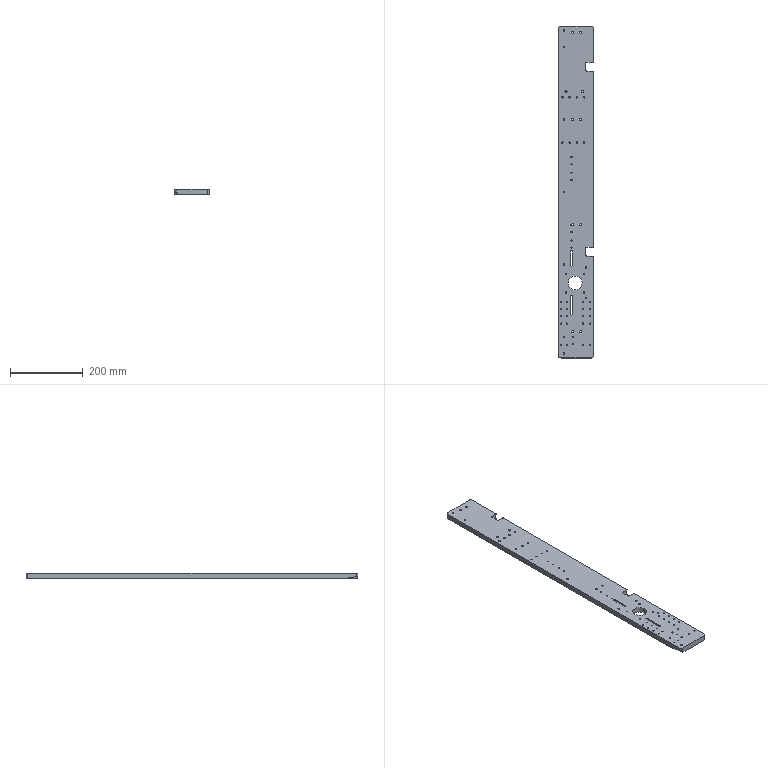Part | STEP file | 1-S938U-100524-003 | 1 solid | 121 faces | box 95 x 915 x 15 mm | volume 1240006 mm3 | cylinder 87 | plane 30 | cone 4 | commonest cylinder face diameters 3.242 x30 4.134 x17 4 x8 4.917 x8 4.4 x6 10 x4